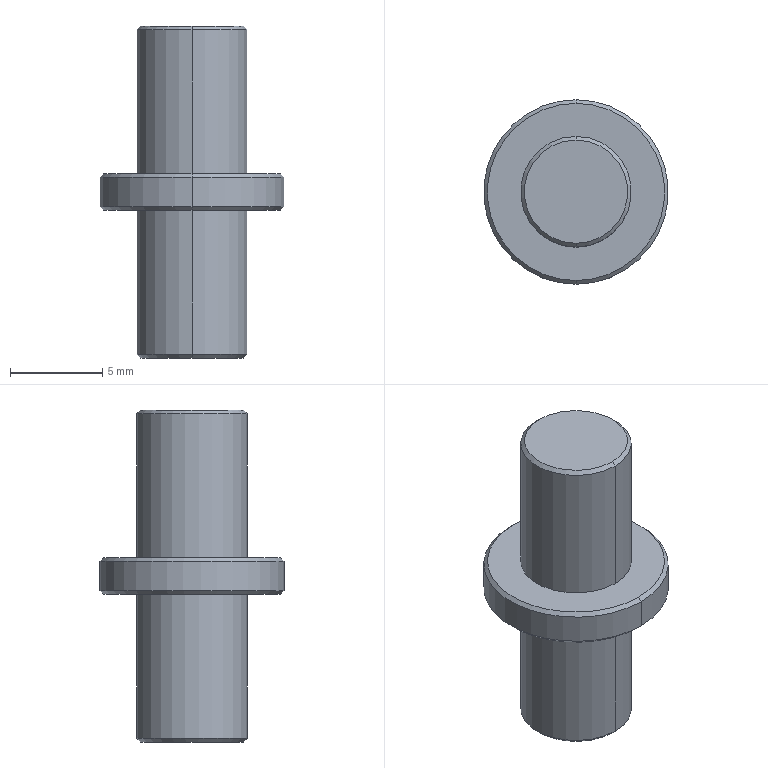Part | STEP file | RJWD-DY-0102_X2_5DE667DC95E8_24 | 1 solid | 18 faces | box 10 x 10 x 18 mm | volume 607.492 mm3 | cone 8 | cylinder 6 | plane 4 | commonest cylinder face diameters 6 x4 10 x2
STEP:
#1=CARTESIAN_POINT('',(0.,0.,0.));
#2=DIRECTION('',(0.,0.,1.));
#3=DIRECTION('',(1.,0.,0.));
#4=AXIS2_PLACEMENT_3D('',#1,#2,#3);
#5=CARTESIAN_POINT('',(-506.773,4252.873,40.144));
#6=VERTEX_POINT('',#5);
#7=CARTESIAN_POINT('',(-506.773,4247.273,40.144));
#8=VERTEX_POINT('',#7);
#9=CARTESIAN_POINT('',(-506.773,4250.073,40.144));
#10=DIRECTION('',(0.,0.,1.));
#11=DIRECTION('',(0.,1.,0.));
#12=AXIS2_PLACEMENT_3D('',#9,#10,#11);
#13=CIRCLE('',#12,2.8);
#14=CARTESIAN_POINT('',(-506.773,4250.073,40.144));
#15=DIRECTION('',(0.,0.,1.));
#16=DIRECTION('',(0.,1.,0.));
#17=AXIS2_PLACEMENT_3D('',#14,#15,#16);
#18=PLANE('',#17);
#19=CARTESIAN_POINT('',(0.,0.));
#20=DIRECTION('',(1.,0.));
#21=AXIS2_PLACEMENT_2D('',#19,#20);
#22=CIRCLE('',#21,2.8);
#23=(GEOMETRIC_REPRESENTATION_CONTEXT(2)PARAMETRIC_REPRESENTATION_CONTEXT()REPRESENTATION_CONTEXT('',''));
#24=DEFINITIONAL_REPRESENTATION('',(#22),#23);
#25=PCURVE('',#18,#24);
#26=CARTESIAN_POINT('',(-506.773,4250.073,40.044));
#27=DIRECTION('',(0.,0.,-1.));
#28=DIRECTION('',(0.,-1.,0.));
#29=AXIS2_PLACEMENT_3D('',#26,#27,#28);
#30=CONICAL_SURFACE('',#29,2.9,0.7854);
#31=CARTESIAN_POINT('',(3.142,-0.1));
#32=DIRECTION('',(-1.,0.));
#33=VECTOR('',#32,1.);
#34=LINE('',#31,#33);
#35=(GEOMETRIC_REPRESENTATION_CONTEXT(2)PARAMETRIC_REPRESENTATION_CONTEXT()REPRESENTATION_CONTEXT('',''));
#36=DEFINITIONAL_REPRESENTATION('',(#34),#35);
#37=PCURVE('',#30,#36);
#38=SURFACE_CURVE('',#13,(#25,#37),.PCURVE_S1.);
#39=EDGE_CURVE('',#6,#8,#38,.T.);
#40=ORIENTED_EDGE('',*,*,#39,.F.);
#41=CARTESIAN_POINT('',(-506.773,4250.073,40.144));
#42=DIRECTION('',(0.,0.,1.));
#43=DIRECTION('',(0.,-1.,0.));
#44=AXIS2_PLACEMENT_3D('',#41,#42,#43);
#45=CIRCLE('',#44,2.8);
#46=CARTESIAN_POINT('',(0.,0.));
#47=DIRECTION('',(-1.,0.));
#48=AXIS2_PLACEMENT_2D('',#46,#47);
#49=CIRCLE('',#48,2.8);
#50=(GEOMETRIC_REPRESENTATION_CONTEXT(2)PARAMETRIC_REPRESENTATION_CONTEXT()REPRESENTATION_CONTEXT('',''));
#51=DEFINITIONAL_REPRESENTATION('',(#49),#50);
#52=PCURVE('',#18,#51);
#53=CARTESIAN_POINT('',(-506.773,4250.073,40.044));
#54=DIRECTION('',(0.,0.,-1.));
#55=DIRECTION('',(0.,-1.,0.));
#56=AXIS2_PLACEMENT_3D('',#53,#54,#55);
#57=CONICAL_SURFACE('',#56,2.9,0.7854);
#58=CARTESIAN_POINT('',(6.283,-0.1));
#59=DIRECTION('',(-1.,0.));
#60=VECTOR('',#59,1.);
#61=LINE('',#58,#60);
#62=(GEOMETRIC_REPRESENTATION_CONTEXT(2)PARAMETRIC_REPRESENTATION_CONTEXT()REPRESENTATION_CONTEXT('',''));
#63=DEFINITIONAL_REPRESENTATION('',(#61),#62);
#64=PCURVE('',#57,#63);
#65=SURFACE_CURVE('',#45,(#52,#64),.PCURVE_S1.);
#66=EDGE_CURVE('',#8,#6,#65,.T.);
#67=ORIENTED_EDGE('',*,*,#66,.F.);
#68=EDGE_LOOP('',(#40,#67));
#69=FACE_BOUND('',#68,.F.);
#70=ADVANCED_FACE('',(#69),#18,.T.);
#71=ORIENTED_EDGE('',*,*,#39,.F.);
#72=CARTESIAN_POINT('',(-506.773,4253.073,39.944));
#73=VERTEX_POINT('',#72);
#74=CARTESIAN_POINT('',(-506.773,4252.873,40.144));
#75=DIRECTION('',(0.,0.7071,-0.7071));
#76=VECTOR('',#75,1.);
#77=LINE('',#74,#76);
#78=CARTESIAN_POINT('',(3.142,-0.1));
#79=DIRECTION('',(0.,1.));
#80=VECTOR('',#79,1.);
#81=LINE('',#78,#80);
#82=(GEOMETRIC_REPRESENTATION_CONTEXT(2)PARAMETRIC_REPRESENTATION_CONTEXT()REPRESENTATION_CONTEXT('',''));
#83=DEFINITIONAL_REPRESENTATION('',(#81),#82);
#84=PCURVE('',#30,#83);
#85=CARTESIAN_POINT('',(3.142,-0.1));
#86=DIRECTION('',(0.,1.));
#87=VECTOR('',#86,1.);
#88=LINE('',#85,#87);
#89=(GEOMETRIC_REPRESENTATION_CONTEXT(2)PARAMETRIC_REPRESENTATION_CONTEXT()REPRESENTATION_CONTEXT('',''));
#90=DEFINITIONAL_REPRESENTATION('',(#88),#89);
#91=PCURVE('',#57,#90);
#92=SURFACE_CURVE('',#77,(#84,#91),.PCURVE_S1.);
#93=EDGE_CURVE('',#6,#73,#92,.T.);
#94=ORIENTED_EDGE('',*,*,#93,.T.);
#95=CARTESIAN_POINT('',(-506.773,4247.073,39.944));
#96=VERTEX_POINT('',#95);
#97=CARTESIAN_POINT('',(-506.773,4250.073,39.944));
#98=DIRECTION('',(0.,0.,1.));
#99=DIRECTION('',(0.,1.,0.));
#100=AXIS2_PLACEMENT_3D('',#97,#98,#99);
#101=CIRCLE('',#100,3.);
#102=CARTESIAN_POINT('',(3.142,0.1));
#103=DIRECTION('',(-1.,0.));
#104=VECTOR('',#103,1.);
#105=LINE('',#102,#104);
#106=(GEOMETRIC_REPRESENTATION_CONTEXT(2)PARAMETRIC_REPRESENTATION_CONTEXT()REPRESENTATION_CONTEXT('',''));
#107=DEFINITIONAL_REPRESENTATION('',(#105),#106);
#108=PCURVE('',#30,#107);
#109=CARTESIAN_POINT('',(-506.773,4250.073,21.244));
#110=DIRECTION('',(0.,0.,1.));
#111=DIRECTION('',(0.,1.,0.));
#112=AXIS2_PLACEMENT_3D('',#109,#110,#111);
#113=CYLINDRICAL_SURFACE('',#112,3.);
#114=CARTESIAN_POINT('',(0.,18.7));
#115=DIRECTION('',(1.,0.));
#116=VECTOR('',#115,1.);
#117=LINE('',#114,#116);
#118=(GEOMETRIC_REPRESENTATION_CONTEXT(2)PARAMETRIC_REPRESENTATION_CONTEXT()REPRESENTATION_CONTEXT('',''));
#119=DEFINITIONAL_REPRESENTATION('',(#117),#118);
#120=PCURVE('',#113,#119);
#121=SURFACE_CURVE('',#101,(#108,#120),.PCURVE_S1.);
#122=EDGE_CURVE('',#73,#96,#121,.T.);
#123=ORIENTED_EDGE('',*,*,#122,.T.);
#124=CARTESIAN_POINT('',(-506.773,4247.273,40.144));
#125=DIRECTION('',(0.,-0.7071,-0.7071));
#126=VECTOR('',#125,1.);
#127=LINE('',#124,#126);
#128=CARTESIAN_POINT('',(0.,-0.1));
#129=DIRECTION('',(0.,1.));
#130=VECTOR('',#129,1.);
#131=LINE('',#128,#130);
#132=(GEOMETRIC_REPRESENTATION_CONTEXT(2)PARAMETRIC_REPRESENTATION_CONTEXT()REPRESENTATION_CONTEXT('',''));
#133=DEFINITIONAL_REPRESENTATION('',(#131),#132);
#134=PCURVE('',#30,#133);
#135=CARTESIAN_POINT('',(6.283,-0.1));
#136=DIRECTION('',(0.,1.));
#137=VECTOR('',#136,1.);
#138=LINE('',#135,#137);
#139=(GEOMETRIC_REPRESENTATION_CONTEXT(2)PARAMETRIC_REPRESENTATION_CONTEXT()REPRESENTATION_CONTEXT('',''));
#140=DEFINITIONAL_REPRESENTATION('',(#138),#139);
#141=PCURVE('',#57,#140);
#142=SURFACE_CURVE('',#127,(#134,#141),.PCURVE_S1.);
#143=EDGE_CURVE('',#8,#96,#142,.T.);
#144=ORIENTED_EDGE('',*,*,#143,.F.);
#145=EDGE_LOOP('',(#71,#94,#123,#144));
#146=FACE_BOUND('',#145,.T.);
#147=ADVANCED_FACE('',(#146),#30,.T.);
#148=ORIENTED_EDGE('',*,*,#66,.F.);
#149=ORIENTED_EDGE('',*,*,#143,.T.);
#150=CARTESIAN_POINT('',(-506.773,4250.073,39.944));
#151=DIRECTION('',(0.,0.,1.));
#152=DIRECTION('',(0.,-1.,0.));
#153=AXIS2_PLACEMENT_3D('',#150,#151,#152);
#154=CIRCLE('',#153,3.);
#155=CARTESIAN_POINT('',(6.283,0.1));
#156=DIRECTION('',(-1.,0.));
#157=VECTOR('',#156,1.);
#158=LINE('',#155,#157);
#159=(GEOMETRIC_REPRESENTATION_CONTEXT(2)PARAMETRIC_REPRESENTATION_CONTEXT()REPRESENTATION_CONTEXT('',''));
#160=DEFINITIONAL_REPRESENTATION('',(#158),#159);
#161=PCURVE('',#57,#160);
#162=CARTESIAN_POINT('',(-506.773,4250.073,21.244));
#163=DIRECTION('',(0.,0.,1.));
#164=DIRECTION('',(0.,1.,0.));
#165=AXIS2_PLACEMENT_3D('',#162,#163,#164);
#166=CYLINDRICAL_SURFACE('',#165,3.);
#167=CARTESIAN_POINT('',(3.142,18.7));
#168=DIRECTION('',(1.,0.));
#169=VECTOR('',#168,1.);
#170=LINE('',#167,#169);
#171=(GEOMETRIC_REPRESENTATION_CONTEXT(2)PARAMETRIC_REPRESENTATION_CONTEXT()REPRESENTATION_CONTEXT('',''));
#172=DEFINITIONAL_REPRESENTATION('',(#170),#171);
#173=PCURVE('',#166,#172);
#174=SURFACE_CURVE('',#154,(#161,#173),.PCURVE_S1.);
#175=EDGE_CURVE('',#96,#73,#174,.T.);
#176=ORIENTED_EDGE('',*,*,#175,.T.);
#177=ORIENTED_EDGE('',*,*,#93,.F.);
#178=EDGE_LOOP('',(#148,#149,#176,#177));
#179=FACE_BOUND('',#178,.T.);
#180=ADVANCED_FACE('',(#179),#57,.T.);
#181=CARTESIAN_POINT('',(-506.773,4253.073,32.144));
#182=VERTEX_POINT('',#181);
#183=CARTESIAN_POINT('',(-506.773,4247.073,32.144));
#184=VERTEX_POINT('',#183);
#185=CARTESIAN_POINT('',(-506.773,4250.073,32.144));
#186=DIRECTION('',(0.,0.,-1.));
#187=DIRECTION('',(0.,1.,0.));
#188=AXIS2_PLACEMENT_3D('',#185,#186,#187);
#189=CIRCLE('',#188,3.);
#190=CARTESIAN_POINT('',(6.283,10.9));
#191=DIRECTION('',(-1.,0.));
#192=VECTOR('',#191,1.);
#193=LINE('',#190,#192);
#194=(GEOMETRIC_REPRESENTATION_CONTEXT(2)PARAMETRIC_REPRESENTATION_CONTEXT()REPRESENTATION_CONTEXT('',''));
#195=DEFINITIONAL_REPRESENTATION('',(#193),#194);
#196=PCURVE('',#166,#195);
#197=CARTESIAN_POINT('',(-506.773,4250.073,32.144));
#198=DIRECTION('',(0.,0.,1.));
#199=DIRECTION('',(0.,1.,0.));
#200=AXIS2_PLACEMENT_3D('',#197,#198,#199);
#201=PLANE('',#200);
#202=CARTESIAN_POINT('',(3.,0.));
#203=CARTESIAN_POINT('',(3.,-5.196));
#204=CARTESIAN_POINT('',(-1.5,-2.598));
#205=CARTESIAN_POINT('',(-6.,0.));
#206=CARTESIAN_POINT('',(-1.5,2.598));
#207=CARTESIAN_POINT('',(3.,5.196));
#208=CARTESIAN_POINT('',(3.,0.));
#209=(BOUNDED_CURVE()B_SPLINE_CURVE(2,(#202,#203,#204,#205,#206,#207,#208),.UNSPECIFIED.,.T.,.F.)B_SPLINE_CURVE_WITH_KNOTS((1,2,2,2,2,1),(-2.094,0.,2.094,4.189,6.283,8.378),.UNSPECIFIED.)CURVE()GEOMETRIC_REPRESENTATION_ITEM()RATIONAL_B_SPLINE_CURVE((1.,0.5,1.,0.5,1.,0.5,1.))REPRESENTATION_ITEM(''));
#210=(GEOMETRIC_REPRESENTATION_CONTEXT(2)PARAMETRIC_REPRESENTATION_CONTEXT()REPRESENTATION_CONTEXT('',''));
#211=DEFINITIONAL_REPRESENTATION('',(#209),#210);
#212=PCURVE('',#201,#211);
#213=SURFACE_CURVE('',#189,(#196,#212),.PCURVE_S1.);
#214=EDGE_CURVE('',#182,#184,#213,.T.);
#215=ORIENTED_EDGE('',*,*,#214,.F.);
#216=CARTESIAN_POINT('',(-506.773,4253.073,32.144));
#217=DIRECTION('',(0.,0.,1.));
#218=VECTOR('',#217,1.);
#219=LINE('',#216,#218);
#220=CARTESIAN_POINT('',(6.283,10.9));
#221=DIRECTION('',(0.,1.));
#222=VECTOR('',#221,1.);
#223=LINE('',#220,#222);
#224=(GEOMETRIC_REPRESENTATION_CONTEXT(2)PARAMETRIC_REPRESENTATION_CONTEXT()REPRESENTATION_CONTEXT('',''));
#225=DEFINITIONAL_REPRESENTATION('',(#223),#224);
#226=PCURVE('',#166,#225);
#227=CARTESIAN_POINT('',(0.,10.9));
#228=DIRECTION('',(0.,1.));
#229=VECTOR('',#228,1.);
#230=LINE('',#227,#229);
#231=(GEOMETRIC_REPRESENTATION_CONTEXT(2)PARAMETRIC_REPRESENTATION_CONTEXT()REPRESENTATION_CONTEXT('',''));
#232=DEFINITIONAL_REPRESENTATION('',(#230),#231);
#233=PCURVE('',#113,#232);
#234=SURFACE_CURVE('',#219,(#226,#233),.PCURVE_S1.);
#235=EDGE_CURVE('',#182,#73,#234,.T.);
#236=ORIENTED_EDGE('',*,*,#235,.T.);
#237=ORIENTED_EDGE('',*,*,#175,.F.);
#238=CARTESIAN_POINT('',(-506.773,4247.073,32.144));
#239=DIRECTION('',(0.,0.,1.));
#240=VECTOR('',#239,1.);
#241=LINE('',#238,#240);
#242=CARTESIAN_POINT('',(3.142,10.9));
#243=DIRECTION('',(0.,1.));
#244=VECTOR('',#243,1.);
#245=LINE('',#242,#244);
#246=(GEOMETRIC_REPRESENTATION_CONTEXT(2)PARAMETRIC_REPRESENTATION_CONTEXT()REPRESENTATION_CONTEXT('',''));
#247=DEFINITIONAL_REPRESENTATION('',(#245),#246);
#248=PCURVE('',#166,#247);
#249=CARTESIAN_POINT('',(3.142,10.9));
#250=DIRECTION('',(0.,1.));
#251=VECTOR('',#250,1.);
#252=LINE('',#249,#251);
#253=(GEOMETRIC_REPRESENTATION_CONTEXT(2)PARAMETRIC_REPRESENTATION_CONTEXT()REPRESENTATION_CONTEXT('',''));
#254=DEFINITIONAL_REPRESENTATION('',(#252),#253);
#255=PCURVE('',#113,#254);
#256=SURFACE_CURVE('',#241,(#248,#255),.PCURVE_S1.);
#257=EDGE_CURVE('',#184,#96,#256,.T.);
#258=ORIENTED_EDGE('',*,*,#257,.F.);
#259=EDGE_LOOP('',(#215,#236,#237,#258));
#260=FACE_BOUND('',#259,.T.);
#261=ADVANCED_FACE('',(#260),#166,.T.);
#262=CARTESIAN_POINT('',(-506.773,4250.073,32.144));
#263=DIRECTION('',(0.,0.,-1.));
#264=DIRECTION('',(0.,-1.,0.));
#265=AXIS2_PLACEMENT_3D('',#262,#263,#264);
#266=CIRCLE('',#265,3.);
#267=CARTESIAN_POINT('',(3.142,10.9));
#268=DIRECTION('',(-1.,0.));
#269=VECTOR('',#268,1.);
#270=LINE('',#267,#269);
#271=(GEOMETRIC_REPRESENTATION_CONTEXT(2)PARAMETRIC_REPRESENTATION_CONTEXT()REPRESENTATION_CONTEXT('',''));
#272=DEFINITIONAL_REPRESENTATION('',(#270),#271);
#273=PCURVE('',#113,#272);
#274=CARTESIAN_POINT('',(-3.,0.));
#275=CARTESIAN_POINT('',(-3.,5.196));
#276=CARTESIAN_POINT('',(1.5,2.598));
#277=CARTESIAN_POINT('',(6.,0.));
#278=CARTESIAN_POINT('',(1.5,-2.598));
#279=CARTESIAN_POINT('',(-3.,-5.196));
#280=CARTESIAN_POINT('',(-3.,0.));
#281=(BOUNDED_CURVE()B_SPLINE_CURVE(2,(#274,#275,#276,#277,#278,#279,#280),.UNSPECIFIED.,.T.,.F.)B_SPLINE_CURVE_WITH_KNOTS((1,2,2,2,2,1),(-2.094,0.,2.094,4.189,6.283,8.378),.UNSPECIFIED.)CURVE()GEOMETRIC_REPRESENTATION_ITEM()RATIONAL_B_SPLINE_CURVE((1.,0.5,1.,0.5,1.,0.5,1.))REPRESENTATION_ITEM(''));
#282=(GEOMETRIC_REPRESENTATION_CONTEXT(2)PARAMETRIC_REPRESENTATION_CONTEXT()REPRESENTATION_CONTEXT('',''));
#283=DEFINITIONAL_REPRESENTATION('',(#281),#282);
#284=PCURVE('',#201,#283);
#285=SURFACE_CURVE('',#266,(#273,#284),.PCURVE_S1.);
#286=EDGE_CURVE('',#184,#182,#285,.T.);
#287=ORIENTED_EDGE('',*,*,#286,.F.);
#288=ORIENTED_EDGE('',*,*,#257,.T.);
#289=ORIENTED_EDGE('',*,*,#122,.F.);
#290=ORIENTED_EDGE('',*,*,#235,.F.);
#291=EDGE_LOOP('',(#287,#288,#289,#290));
#292=FACE_BOUND('',#291,.T.);
#293=ADVANCED_FACE('',(#292),#113,.T.);
#294=CARTESIAN_POINT('',(-506.773,4254.873,32.144));
#295=VERTEX_POINT('',#294);
#296=CARTESIAN_POINT('',(-506.773,4245.273,32.144));
#297=VERTEX_POINT('',#296);
#298=CARTESIAN_POINT('',(-506.773,4250.073,32.144));
#299=DIRECTION('',(0.,0.,1.));
#300=DIRECTION('',(0.,1.,0.));
#301=AXIS2_PLACEMENT_3D('',#298,#299,#300);
#302=CIRCLE('',#301,4.8);
#303=CARTESIAN_POINT('',(0.,0.));
#304=DIRECTION('',(1.,0.));
#305=AXIS2_PLACEMENT_2D('',#303,#304);
#306=CIRCLE('',#305,4.8);
#307=(GEOMETRIC_REPRESENTATION_CONTEXT(2)PARAMETRIC_REPRESENTATION_CONTEXT()REPRESENTATION_CONTEXT('',''));
#308=DEFINITIONAL_REPRESENTATION('',(#306),#307);
#309=PCURVE('',#201,#308);
#310=CARTESIAN_POINT('',(-506.773,4250.073,32.044));
#311=DIRECTION('',(0.,0.,-1.));
#312=DIRECTION('',(0.,-1.,0.));
#313=AXIS2_PLACEMENT_3D('',#310,#311,#312);
#314=CONICAL_SURFACE('',#313,4.9,0.7854);
#315=CARTESIAN_POINT('',(3.142,-0.1));
#316=DIRECTION('',(-1.,0.));
#317=VECTOR('',#316,1.);
#318=LINE('',#315,#317);
#319=(GEOMETRIC_REPRESENTATION_CONTEXT(2)PARAMETRIC_REPRESENTATION_CONTEXT()REPRESENTATION_CONTEXT('',''));
#320=DEFINITIONAL_REPRESENTATION('',(#318),#319);
#321=PCURVE('',#314,#320);
#322=SURFACE_CURVE('',#302,(#309,#321),.PCURVE_S1.);
#323=EDGE_CURVE('',#295,#297,#322,.T.);
#324=ORIENTED_EDGE('',*,*,#323,.F.);
#325=CARTESIAN_POINT('',(-506.773,4250.073,32.144));
#326=DIRECTION('',(0.,0.,1.));
#327=DIRECTION('',(0.,-1.,0.));
#328=AXIS2_PLACEMENT_3D('',#325,#326,#327);
#329=CIRCLE('',#328,4.8);
#330=CARTESIAN_POINT('',(0.,0.));
#331=DIRECTION('',(-1.,0.));
#332=AXIS2_PLACEMENT_2D('',#330,#331);
#333=CIRCLE('',#332,4.8);
#334=(GEOMETRIC_REPRESENTATION_CONTEXT(2)PARAMETRIC_REPRESENTATION_CONTEXT()REPRESENTATION_CONTEXT('',''));
#335=DEFINITIONAL_REPRESENTATION('',(#333),#334);
#336=PCURVE('',#201,#335);
#337=CARTESIAN_POINT('',(-506.773,4250.073,32.044));
#338=DIRECTION('',(0.,0.,-1.));
#339=DIRECTION('',(0.,-1.,0.));
#340=AXIS2_PLACEMENT_3D('',#337,#338,#339);
#341=CONICAL_SURFACE('',#340,4.9,0.7854);
#342=CARTESIAN_POINT('',(6.283,-0.1));
#343=DIRECTION('',(-1.,0.));
#344=VECTOR('',#343,1.);
#345=LINE('',#342,#344);
#346=(GEOMETRIC_REPRESENTATION_CONTEXT(2)PARAMETRIC_REPRESENTATION_CONTEXT()REPRESENTATION_CONTEXT('',''));
#347=DEFINITIONAL_REPRESENTATION('',(#345),#346);
#348=PCURVE('',#341,#347);
#349=SURFACE_CURVE('',#329,(#336,#348),.PCURVE_S1.);
#350=EDGE_CURVE('',#297,#295,#349,.T.);
#351=ORIENTED_EDGE('',*,*,#350,.F.);
#352=EDGE_LOOP('',(#324,#351));
#353=FACE_BOUND('',#352,.F.);
#354=ORIENTED_EDGE('',*,*,#214,.F.);
#355=ORIENTED_EDGE('',*,*,#286,.F.);
#356=EDGE_LOOP('',(#354,#355));
#357=FACE_BOUND('',#356,.F.);
#358=ADVANCED_FACE('',(#353,#357),#201,.T.);
#359=ORIENTED_EDGE('',*,*,#323,.F.);
#360=CARTESIAN_POINT('',(-506.773,4255.073,31.944));
#361=VERTEX_POINT('',#360);
#362=CARTESIAN_POINT('',(-506.773,4254.873,32.144));
#363=DIRECTION('',(0.,0.7071,-0.7071));
#364=VECTOR('',#363,1.);
#365=LINE('',#362,#364);
#366=CARTESIAN_POINT('',(3.142,-0.1));
#367=DIRECTION('',(0.,1.));
#368=VECTOR('',#367,1.);
#369=LINE('',#366,#368);
#370=(GEOMETRIC_REPRESENTATION_CONTEXT(2)PARAMETRIC_REPRESENTATION_CONTEXT()REPRESENTATION_CONTEXT('',''));
#371=DEFINITIONAL_REPRESENTATION('',(#369),#370);
#372=PCURVE('',#314,#371);
#373=CARTESIAN_POINT('',(3.142,-0.1));
#374=DIRECTION('',(0.,1.));
#375=VECTOR('',#374,1.);
#376=LINE('',#373,#375);
#377=(GEOMETRIC_REPRESENTATION_CONTEXT(2)PARAMETRIC_REPRESENTATION_CONTEXT()REPRESENTATION_CONTEXT('',''));
#378=DEFINITIONAL_REPRESENTATION('',(#376),#377);
#379=PCURVE('',#341,#378);
#380=SURFACE_CURVE('',#365,(#372,#379),.PCURVE_S1.);
#381=EDGE_CURVE('',#295,#361,#380,.T.);
#382=ORIENTED_EDGE('',*,*,#381,.T.);
#383=CARTESIAN_POINT('',(-506.773,4245.073,31.944));
#384=VERTEX_POINT('',#383);
#385=CARTESIAN_POINT('',(-506.773,4250.073,31.944));
#386=DIRECTION('',(0.,0.,1.));
#387=DIRECTION('',(0.,1.,0.));
#388=AXIS2_PLACEMENT_3D('',#385,#386,#387);
#389=CIRCLE('',#388,5.);
#390=CARTESIAN_POINT('',(3.142,0.1));
#391=DIRECTION('',(-1.,0.));
#392=VECTOR('',#391,1.);
#393=LINE('',#390,#392);
#394=(GEOMETRIC_REPRESENTATION_CONTEXT(2)PARAMETRIC_REPRESENTATION_CONTEXT()REPRESENTATION_CONTEXT('',''));
#395=DEFINITIONAL_REPRESENTATION('',(#393),#394);
#396=PCURVE('',#314,#395);
#397=CARTESIAN_POINT('',(-506.773,4250.073,21.244));
#398=DIRECTION('',(0.,0.,1.));
#399=DIRECTION('',(0.,1.,0.));
#400=AXIS2_PLACEMENT_3D('',#397,#398,#399);
#401=CYLINDRICAL_SURFACE('',#400,5.);
#402=CARTESIAN_POINT('',(0.,10.7));
#403=DIRECTION('',(1.,0.));
#404=VECTOR('',#403,1.);
#405=LINE('',#402,#404);
#406=(GEOMETRIC_REPRESENTATION_CONTEXT(2)PARAMETRIC_REPRESENTATION_CONTEXT()REPRESENTATION_CONTEXT('',''));
#407=DEFINITIONAL_REPRESENTATION('',(#405),#406);
#408=PCURVE('',#401,#407);
#409=SURFACE_CURVE('',#389,(#396,#408),.PCURVE_S1.);
#410=EDGE_CURVE('',#361,#384,#409,.T.);
#411=ORIENTED_EDGE('',*,*,#410,.T.);
#412=CARTESIAN_POINT('',(-506.773,4245.273,32.144));
#413=DIRECTION('',(0.,-0.7071,-0.7071));
#414=VECTOR('',#413,1.);
#415=LINE('',#412,#414);
#416=CARTESIAN_POINT('',(0.,-0.1));
#417=DIRECTION('',(0.,1.));
#418=VECTOR('',#417,1.);
#419=LINE('',#416,#418);
#420=(GEOMETRIC_REPRESENTATION_CONTEXT(2)PARAMETRIC_REPRESENTATION_CONTEXT()REPRESENTATION_CONTEXT('',''));
#421=DEFINITIONAL_REPRESENTATION('',(#419),#420);
#422=PCURVE('',#314,#421);
#423=CARTESIAN_POINT('',(6.283,-0.1));
#424=DIRECTION('',(0.,1.));
#425=VECTOR('',#424,1.);
#426=LINE('',#423,#425);
#427=(GEOMETRIC_REPRESENTATION_CONTEXT(2)PARAMETRIC_REPRESENTATION_CONTEXT()REPRESENTATION_CONTEXT('',''));
#428=DEFINITIONAL_REPRESENTATION('',(#426),#427);
#429=PCURVE('',#341,#428);
#430=SURFACE_CURVE('',#415,(#422,#429),.PCURVE_S1.);
#431=EDGE_CURVE('',#297,#384,#430,.T.);
#432=ORIENTED_EDGE('',*,*,#431,.F.);
#433=EDGE_LOOP('',(#359,#382,#411,#432));
#434=FACE_BOUND('',#433,.T.);
#435=ADVANCED_FACE('',(#434),#314,.T.);
#436=ORIENTED_EDGE('',*,*,#350,.F.);
#437=ORIENTED_EDGE('',*,*,#431,.T.);
#438=CARTESIAN_POINT('',(-506.773,4250.073,31.944));
#439=DIRECTION('',(0.,0.,1.));
#440=DIRECTION('',(0.,-1.,0.));
#441=AXIS2_PLACEMENT_3D('',#438,#439,#440);
#442=CIRCLE('',#441,5.);
#443=CARTESIAN_POINT('',(6.283,0.1));
#444=DIRECTION('',(-1.,0.));
#445=VECTOR('',#444,1.);
#446=LINE('',#443,#445);
#447=(GEOMETRIC_REPRESENTATION_CONTEXT(2)PARAMETRIC_REPRESENTATION_CONTEXT()REPRESENTATION_CONTEXT('',''));
#448=DEFINITIONAL_REPRESENTATION('',(#446),#447);
#449=PCURVE('',#341,#448);
#450=CARTESIAN_POINT('',(-506.773,4250.073,21.244));
#451=DIRECTION('',(0.,0.,1.));
#452=DIRECTION('',(0.,1.,0.));
#453=AXIS2_PLACEMENT_3D('',#450,#451,#452);
#454=CYLINDRICAL_SURFACE('',#453,5.);
#455=CARTESIAN_POINT('',(3.142,10.7));
#456=DIRECTION('',(1.,0.));
#457=VECTOR('',#456,1.);
#458=LINE('',#455,#457);
#459=(GEOMETRIC_REPRESENTATION_CONTEXT(2)PARAMETRIC_REPRESENTATION_CONTEXT()REPRESENTATION_CONTEXT('',''));
#460=DEFINITIONAL_REPRESENTATION('',(#458),#459);
#461=PCURVE('',#454,#460);
#462=SURFACE_CURVE('',#442,(#449,#461),.PCURVE_S1.);
#463=EDGE_CURVE('',#384,#361,#462,.T.);
#464=ORIENTED_EDGE('',*,*,#463,.T.);
#465=ORIENTED_EDGE('',*,*,#381,.F.);
#466=EDGE_LOOP('',(#436,#437,#464,#465));
#467=FACE_BOUND('',#466,.T.);
#468=ADVANCED_FACE('',(#467),#341,.T.);
#469=ORIENTED_EDGE('',*,*,#463,.F.);
#470=CARTESIAN_POINT('',(-506.773,4245.073,30.344));
#471=VERTEX_POINT('',#470);
#472=CARTESIAN_POINT('',(-506.773,4245.073,30.344));
#473=DIRECTION('',(0.,0.,1.));
#474=VECTOR('',#473,1.);
#475=LINE('',#472,#474);
#476=CARTESIAN_POINT('',(3.142,9.1));
#477=DIRECTION('',(0.,1.));
#478=VECTOR('',#477,1.);
#479=LINE('',#476,#478);
#480=(GEOMETRIC_REPRESENTATION_CONTEXT(2)PARAMETRIC_REPRESENTATION_CONTEXT()REPRESENTATION_CONTEXT('',''));
#481=DEFINITIONAL_REPRESENTATION('',(#479),#480);
#482=PCURVE('',#454,#481);
#483=CARTESIAN_POINT('',(3.142,9.1));
#484=DIRECTION('',(0.,1.));
#485=VECTOR('',#484,1.);
#486=LINE('',#483,#485);
#487=(GEOMETRIC_REPRESENTATION_CONTEXT(2)PARAMETRIC_REPRESENTATION_CONTEXT()REPRESENTATION_CONTEXT('',''));
#488=DEFINITIONAL_REPRESENTATION('',(#486),#487);
#489=PCURVE('',#401,#488);
#490=SURFACE_CURVE('',#475,(#482,#489),.PCURVE_S1.);
#491=EDGE_CURVE('',#471,#384,#490,.T.);
#492=ORIENTED_EDGE('',*,*,#491,.F.);
#493=CARTESIAN_POINT('',(-506.773,4255.073,30.344));
#494=VERTEX_POINT('',#493);
#495=CARTESIAN_POINT('',(-506.773,4250.073,30.344));
#496=DIRECTION('',(0.,0.,-1.));
#497=DIRECTION('',(0.,1.,0.));
#498=AXIS2_PLACEMENT_3D('',#495,#496,#497);
#499=CIRCLE('',#498,5.);
#500=CARTESIAN_POINT('',(6.283,9.1));
#501=DIRECTION('',(-1.,0.));
#502=VECTOR('',#501,1.);
#503=LINE('',#500,#502);
#504=(GEOMETRIC_REPRESENTATION_CONTEXT(2)PARAMETRIC_REPRESENTATION_CONTEXT()REPRESENTATION_CONTEXT('',''));
#505=DEFINITIONAL_REPRESENTATION('',(#503),#504);
#506=PCURVE('',#454,#505);
#507=CARTESIAN_POINT('',(-506.773,4250.073,30.244));
#508=DIRECTION('',(0.,0.,1.));
#509=DIRECTION('',(0.,-1.,0.));
#510=AXIS2_PLACEMENT_3D('',#507,#508,#509);
#511=CONICAL_SURFACE('',#510,4.9,0.7854);
#512=CARTESIAN_POINT('',(3.142,0.1));
#513=DIRECTION('',(-1.,0.));
#514=VECTOR('',#513,1.);
#515=LINE('',#512,#514);
#516=(GEOMETRIC_REPRESENTATION_CONTEXT(2)PARAMETRIC_REPRESENTATION_CONTEXT()REPRESENTATION_CONTEXT('',''));
#517=DEFINITIONAL_REPRESENTATION('',(#515),#516);
#518=PCURVE('',#511,#517);
#519=SURFACE_CURVE('',#499,(#506,#518),.PCURVE_S1.);
#520=EDGE_CURVE('',#494,#471,#519,.T.);
#521=ORIENTED_EDGE('',*,*,#520,.F.);
#522=CARTESIAN_POINT('',(-506.773,4255.073,30.344));
#523=DIRECTION('',(0.,0.,1.));
#524=VECTOR('',#523,1.);
#525=LINE('',#522,#524);
#526=CARTESIAN_POINT('',(6.283,9.1));
#527=DIRECTION('',(0.,1.));
#528=VECTOR('',#527,1.);
#529=LINE('',#526,#528);
#530=(GEOMETRIC_REPRESENTATION_CONTEXT(2)PARAMETRIC_REPRESENTATION_CONTEXT()REPRESENTATION_CONTEXT('',''));
#531=DEFINITIONAL_REPRESENTATION('',(#529),#530);
#532=PCURVE('',#454,#531);
#533=CARTESIAN_POINT('',(0.,9.1));
#534=DIRECTION('',(0.,1.));
#535=VECTOR('',#534,1.);
#536=LINE('',#533,#535);
#537=(GEOMETRIC_REPRESENTATION_CONTEXT(2)PARAMETRIC_REPRESENTATION_CONTEXT()REPRESENTATION_CONTEXT('',''));
#538=DEFINITIONAL_REPRESENTATION('',(#536),#537);
#539=PCURVE('',#401,#538);
#540=SURFACE_CURVE('',#525,(#532,#539),.PCURVE_S1.);
#541=EDGE_CURVE('',#494,#361,#540,.T.);
#542=ORIENTED_EDGE('',*,*,#541,.T.);
#543=EDGE_LOOP('',(#469,#492,#521,#542));
#544=FACE_BOUND('',#543,.T.);
#545=ADVANCED_FACE('',(#544),#454,.T.);
#546=ORIENTED_EDGE('',*,*,#410,.F.);
#547=ORIENTED_EDGE('',*,*,#541,.F.);
#548=CARTESIAN_POINT('',(-506.773,4250.073,30.344));
#549=DIRECTION('',(0.,0.,-1.));
#550=DIRECTION('',(0.,-1.,0.));
#551=AXIS2_PLACEMENT_3D('',#548,#549,#550);
#552=CIRCLE('',#551,5.);
#553=CARTESIAN_POINT('',(3.142,9.1));
#554=DIRECTION('',(-1.,0.));
#555=VECTOR('',#554,1.);
#556=LINE('',#553,#555);
#557=(GEOMETRIC_REPRESENTATION_CONTEXT(2)PARAMETRIC_REPRESENTATION_CONTEXT()REPRESENTATION_CONTEXT('',''));
#558=DEFINITIONAL_REPRESENTATION('',(#556),#557);
#559=PCURVE('',#401,#558);
#560=CARTESIAN_POINT('',(-506.773,4250.073,30.244));
#561=DIRECTION('',(0.,0.,1.));
#562=DIRECTION('',(0.,-1.,0.));
#563=AXIS2_PLACEMENT_3D('',#560,#561,#562);
#564=CONICAL_SURFACE('',#563,4.9,0.7854);
#565=CARTESIAN_POINT('',(6.283,0.1));
#566=DIRECTION('',(-1.,0.));
#567=VECTOR('',#566,1.);
#568=LINE('',#565,#567);
#569=(GEOMETRIC_REPRESENTATION_CONTEXT(2)PARAMETRIC_REPRESENTATION_CONTEXT()REPRESENTATION_CONTEXT('',''));
#570=DEFINITIONAL_REPRESENTATION('',(#568),#569);
#571=PCURVE('',#564,#570);
#572=SURFACE_CURVE('',#552,(#559,#571),.PCURVE_S1.);
#573=EDGE_CURVE('',#471,#494,#572,.T.);
#574=ORIENTED_EDGE('',*,*,#573,.F.);
#575=ORIENTED_EDGE('',*,*,#491,.T.);
#576=EDGE_LOOP('',(#546,#547,#574,#575));
#577=FACE_BOUND('',#576,.T.);
#578=ADVANCED_FACE('',(#577),#401,.T.);
#579=ORIENTED_EDGE('',*,*,#573,.T.);
#580=CARTESIAN_POINT('',(-506.773,4254.873,30.144));
#581=VERTEX_POINT('',#580);
#582=CARTESIAN_POINT('',(-506.773,4255.073,30.344));
#583=DIRECTION('',(0.,-0.7071,-0.7071));
#584=VECTOR('',#583,1.);
#585=LINE('',#582,#584);
#586=CARTESIAN_POINT('',(3.142,0.1));
#587=DIRECTION('',(0.,-1.));
#588=VECTOR('',#587,1.);
#589=LINE('',#586,#588);
#590=(GEOMETRIC_REPRESENTATION_CONTEXT(2)PARAMETRIC_REPRESENTATION_CONTEXT()REPRESENTATION_CONTEXT('',''));
#591=DEFINITIONAL_REPRESENTATION('',(#589),#590);
#592=PCURVE('',#564,#591);
#593=CARTESIAN_POINT('',(3.142,0.1));
#594=DIRECTION('',(0.,-1.));
#595=VECTOR('',#594,1.);
#596=LINE('',#593,#595);
#597=(GEOMETRIC_REPRESENTATION_CONTEXT(2)PARAMETRIC_REPRESENTATION_CONTEXT()REPRESENTATION_CONTEXT('',''));
#598=DEFINITIONAL_REPRESENTATION('',(#596),#597);
#599=PCURVE('',#511,#598);
#600=SURFACE_CURVE('',#585,(#592,#599),.PCURVE_S1.);
#601=EDGE_CURVE('',#494,#581,#600,.T.);
#602=ORIENTED_EDGE('',*,*,#601,.T.);
#603=CARTESIAN_POINT('',(-506.773,4245.273,30.144));
#604=VERTEX_POINT('',#603);
#605=CARTESIAN_POINT('',(-506.773,4250.073,30.144));
#606=DIRECTION('',(0.,0.,-1.));
#607=DIRECTION('',(0.,-1.,0.));
#608=AXIS2_PLACEMENT_3D('',#605,#606,#607);
#609=CIRCLE('',#608,4.8);
#610=CARTESIAN_POINT('',(6.283,-0.1));
#611=DIRECTION('',(-1.,0.));
#612=VECTOR('',#611,1.);
#613=LINE('',#610,#612);
#614=(GEOMETRIC_REPRESENTATION_CONTEXT(2)PARAMETRIC_REPRESENTATION_CONTEXT()REPRESENTATION_CONTEXT('',''));
#615=DEFINITIONAL_REPRESENTATION('',(#613),#614);
#616=PCURVE('',#564,#615);
#617=CARTESIAN_POINT('',(-506.773,4250.073,30.144));
#618=DIRECTION('',(0.,0.,1.));
#619=DIRECTION('',(0.,1.,0.));
#620=AXIS2_PLACEMENT_3D('',#617,#618,#619);
#621=PLANE('',#620);
#622=CARTESIAN_POINT('',(-4.8,0.));
#623=CARTESIAN_POINT('',(-4.8,8.314));
#624=CARTESIAN_POINT('',(2.4,4.157));
#625=CARTESIAN_POINT('',(9.6,0.));
#626=CARTESIAN_POINT('',(2.4,-4.157));
#627=CARTESIAN_POINT('',(-4.8,-8.314));
#628=CARTESIAN_POINT('',(-4.8,0.));
#629=(BOUNDED_CURVE()B_SPLINE_CURVE(2,(#622,#623,#624,#625,#626,#627,#628),.UNSPECIFIED.,.T.,.F.)B_SPLINE_CURVE_WITH_KNOTS((1,2,2,2,2,1),(-2.094,0.,2.094,4.189,6.283,8.378),.UNSPECIFIED.)CURVE()GEOMETRIC_REPRESENTATION_ITEM()RATIONAL_B_SPLINE_CURVE((1.,0.5,1.,0.5,1.,0.5,1.))REPRESENTATION_ITEM(''));
#630=(GEOMETRIC_REPRESENTATION_CONTEXT(2)PARAMETRIC_REPRESENTATION_CONTEXT()REPRESENTATION_CONTEXT('',''));
#631=DEFINITIONAL_REPRESENTATION('',(#629),#630);
#632=PCURVE('',#621,#631);
#633=SURFACE_CURVE('',#609,(#616,#632),.PCURVE_S1.);
#634=EDGE_CURVE('',#604,#581,#633,.T.);
#635=ORIENTED_EDGE('',*,*,#634,.F.);
#636=CARTESIAN_POINT('',(-506.773,4245.073,30.344));
#637=DIRECTION('',(0.,0.7071,-0.7071));
#638=VECTOR('',#637,1.);
#639=LINE('',#636,#638);
#640=CARTESIAN_POINT('',(6.283,0.1));
#641=DIRECTION('',(0.,-1.));
#642=VECTOR('',#641,1.);
#643=LINE('',#640,#642);
#644=(GEOMETRIC_REPRESENTATION_CONTEXT(2)PARAMETRIC_REPRESENTATION_CONTEXT()REPRESENTATION_CONTEXT('',''));
#645=DEFINITIONAL_REPRESENTATION('',(#643),#644);
#646=PCURVE('',#564,#645);
#647=CARTESIAN_POINT('',(0.,0.1));
#648=DIRECTION('',(0.,-1.));
#649=VECTOR('',#648,1.);
#650=LINE('',#647,#649);
#651=(GEOMETRIC_REPRESENTATION_CONTEXT(2)PARAMETRIC_REPRESENTATION_CONTEXT()REPRESENTATION_CONTEXT('',''));
#652=DEFINITIONAL_REPRESENTATION('',(#650),#651);
#653=PCURVE('',#511,#652);
#654=SURFACE_CURVE('',#639,(#646,#653),.PCURVE_S1.);
#655=EDGE_CURVE('',#471,#604,#654,.T.);
#656=ORIENTED_EDGE('',*,*,#655,.F.);
#657=EDGE_LOOP('',(#579,#602,#635,#656));
#658=FACE_BOUND('',#657,.T.);
#659=ADVANCED_FACE('',(#658),#564,.T.);
#660=ORIENTED_EDGE('',*,*,#520,.T.);
#661=ORIENTED_EDGE('',*,*,#655,.T.);
#662=CARTESIAN_POINT('',(-506.773,4250.073,30.144));
#663=DIRECTION('',(0.,0.,-1.));
#664=DIRECTION('',(0.,1.,0.));
#665=AXIS2_PLACEMENT_3D('',#662,#663,#664);
#666=CIRCLE('',#665,4.8);
#667=CARTESIAN_POINT('',(3.142,-0.1));
#668=DIRECTION('',(-1.,0.));
#669=VECTOR('',#668,1.);
#670=LINE('',#667,#669);
#671=(GEOMETRIC_REPRESENTATION_CONTEXT(2)PARAMETRIC_REPRESENTATION_CONTEXT()REPRESENTATION_CONTEXT('',''));
#672=DEFINITIONAL_REPRESENTATION('',(#670),#671);
#673=PCURVE('',#511,#672);
#674=CARTESIAN_POINT('',(4.8,0.));
#675=CARTESIAN_POINT('',(4.8,-8.314));
#676=CARTESIAN_POINT('',(-2.4,-4.157));
#677=CARTESIAN_POINT('',(-9.6,0.));
#678=CARTESIAN_POINT('',(-2.4,4.157));
#679=CARTESIAN_POINT('',(4.8,8.314));
#680=CARTESIAN_POINT('',(4.8,0.));
#681=(BOUNDED_CURVE()B_SPLINE_CURVE(2,(#674,#675,#676,#677,#678,#679,#680),.UNSPECIFIED.,.T.,.F.)B_SPLINE_CURVE_WITH_KNOTS((1,2,2,2,2,1),(-2.094,0.,2.094,4.189,6.283,8.378),.UNSPECIFIED.)CURVE()GEOMETRIC_REPRESENTATION_ITEM()RATIONAL_B_SPLINE_CURVE((1.,0.5,1.,0.5,1.,0.5,1.))REPRESENTATION_ITEM(''));
#682=(GEOMETRIC_REPRESENTATION_CONTEXT(2)PARAMETRIC_REPRESENTATION_CONTEXT()REPRESENTATION_CONTEXT('',''));
#683=DEFINITIONAL_REPRESENTATION('',(#681),#682);
#684=PCURVE('',#621,#683);
#685=SURFACE_CURVE('',#666,(#673,#684),.PCURVE_S1.);
#686=EDGE_CURVE('',#581,#604,#685,.T.);
#687=ORIENTED_EDGE('',*,*,#686,.F.);
#688=ORIENTED_EDGE('',*,*,#601,.F.);
#689=EDGE_LOOP('',(#660,#661,#687,#688));
#690=FACE_BOUND('',#689,.T.);
#691=ADVANCED_FACE('',(#690),#511,.T.);
#692=ORIENTED_EDGE('',*,*,#634,.F.);
#693=ORIENTED_EDGE('',*,*,#686,.F.);
#694=EDGE_LOOP('',(#692,#693));
#695=FACE_BOUND('',#694,.F.);
#696=CARTESIAN_POINT('',(-506.773,4253.073,30.144));
#697=VERTEX_POINT('',#696);
#698=CARTESIAN_POINT('',(-506.773,4247.073,30.144));
#699=VERTEX_POINT('',#698);
#700=CARTESIAN_POINT('',(-506.773,4250.073,30.144));
#701=DIRECTION('',(0.,0.,1.));
#702=DIRECTION('',(0.,1.,0.));
#703=AXIS2_PLACEMENT_3D('',#700,#701,#702);
#704=CIRCLE('',#703,3.);
#705=CARTESIAN_POINT('',(0.,0.));
#706=DIRECTION('',(1.,0.));
#707=AXIS2_PLACEMENT_2D('',#705,#706);
#708=CIRCLE('',#707,3.);
#709=(GEOMETRIC_REPRESENTATION_CONTEXT(2)PARAMETRIC_REPRESENTATION_CONTEXT()REPRESENTATION_CONTEXT('',''));
#710=DEFINITIONAL_REPRESENTATION('',(#708),#709);
#711=PCURVE('',#621,#710);
#712=CARTESIAN_POINT('',(-506.773,4250.073,21.244));
#713=DIRECTION('',(0.,0.,1.));
#714=DIRECTION('',(0.,1.,0.));
#715=AXIS2_PLACEMENT_3D('',#712,#713,#714);
#716=CYLINDRICAL_SURFACE('',#715,3.);
#717=CARTESIAN_POINT('',(0.,8.9));
#718=DIRECTION('',(1.,0.));
#719=VECTOR('',#718,1.);
#720=LINE('',#717,#719);
#721=(GEOMETRIC_REPRESENTATION_CONTEXT(2)PARAMETRIC_REPRESENTATION_CONTEXT()REPRESENTATION_CONTEXT('',''));
#722=DEFINITIONAL_REPRESENTATION('',(#720),#721);
#723=PCURVE('',#716,#722);
#724=SURFACE_CURVE('',#704,(#711,#723),.PCURVE_S1.);
#725=EDGE_CURVE('',#697,#699,#724,.T.);
#726=ORIENTED_EDGE('',*,*,#725,.F.);
#727=CARTESIAN_POINT('',(-506.773,4250.073,30.144));
#728=DIRECTION('',(0.,0.,1.));
#729=DIRECTION('',(0.,-1.,0.));
#730=AXIS2_PLACEMENT_3D('',#727,#728,#729);
#731=CIRCLE('',#730,3.);
#732=CARTESIAN_POINT('',(0.,0.));
#733=DIRECTION('',(-1.,0.));
#734=AXIS2_PLACEMENT_2D('',#732,#733);
#735=CIRCLE('',#734,3.);
#736=(GEOMETRIC_REPRESENTATION_CONTEXT(2)PARAMETRIC_REPRESENTATION_CONTEXT()REPRESENTATION_CONTEXT('',''));
#737=DEFINITIONAL_REPRESENTATION('',(#735),#736);
#738=PCURVE('',#621,#737);
#739=CARTESIAN_POINT('',(-506.773,4250.073,21.244));
#740=DIRECTION('',(0.,0.,1.));
#741=DIRECTION('',(0.,1.,0.));
#742=AXIS2_PLACEMENT_3D('',#739,#740,#741);
#743=CYLINDRICAL_SURFACE('',#742,3.);
#744=CARTESIAN_POINT('',(3.142,8.9));
#745=DIRECTION('',(1.,0.));
#746=VECTOR('',#745,1.);
#747=LINE('',#744,#746);
#748=(GEOMETRIC_REPRESENTATION_CONTEXT(2)PARAMETRIC_REPRESENTATION_CONTEXT()REPRESENTATION_CONTEXT('',''));
#749=DEFINITIONAL_REPRESENTATION('',(#747),#748);
#750=PCURVE('',#743,#749);
#751=SURFACE_CURVE('',#731,(#738,#750),.PCURVE_S1.);
#752=EDGE_CURVE('',#699,#697,#751,.T.);
#753=ORIENTED_EDGE('',*,*,#752,.F.);
#754=EDGE_LOOP('',(#726,#753));
#755=FACE_BOUND('',#754,.F.);
#756=ADVANCED_FACE('',(#695,#755),#621,.F.);
#757=ORIENTED_EDGE('',*,*,#725,.F.);
#758=CARTESIAN_POINT('',(-506.773,4253.073,22.344));
#759=VERTEX_POINT('',#758);
#760=CARTESIAN_POINT('',(-506.773,4253.073,22.344));
#761=DIRECTION('',(0.,0.,1.));
#762=VECTOR('',#761,1.);
#763=LINE('',#760,#762);
#764=CARTESIAN_POINT('',(0.,1.1));
#765=DIRECTION('',(0.,1.));
#766=VECTOR('',#765,1.);
#767=LINE('',#764,#766);
#768=(GEOMETRIC_REPRESENTATION_CONTEXT(2)PARAMETRIC_REPRESENTATION_CONTEXT()REPRESENTATION_CONTEXT('',''));
#769=DEFINITIONAL_REPRESENTATION('',(#767),#768);
#770=PCURVE('',#716,#769);
#771=CARTESIAN_POINT('',(6.283,1.1));
#772=DIRECTION('',(0.,1.));
#773=VECTOR('',#772,1.);
#774=LINE('',#771,#773);
#775=(GEOMETRIC_REPRESENTATION_CONTEXT(2)PARAMETRIC_REPRESENTATION_CONTEXT()REPRESENTATION_CONTEXT('',''));
#776=DEFINITIONAL_REPRESENTATION('',(#774),#775);
#777=PCURVE('',#743,#776);
#778=SURFACE_CURVE('',#763,(#770,#777),.PCURVE_S1.);
#779=EDGE_CURVE('',#759,#697,#778,.T.);
#780=ORIENTED_EDGE('',*,*,#779,.F.);
#781=CARTESIAN_POINT('',(-506.773,4247.073,22.344));
#782=VERTEX_POINT('',#781);
#783=CARTESIAN_POINT('',(-506.773,4250.073,22.344));
#784=DIRECTION('',(0.,0.,-1.));
#785=DIRECTION('',(0.,-1.,0.));
#786=AXIS2_PLACEMENT_3D('',#783,#784,#785);
#787=CIRCLE('',#786,3.);
#788=CARTESIAN_POINT('',(3.142,1.1));
#789=DIRECTION('',(-1.,0.));
#790=VECTOR('',#789,1.);
#791=LINE('',#788,#790);
#792=(GEOMETRIC_REPRESENTATION_CONTEXT(2)PARAMETRIC_REPRESENTATION_CONTEXT()REPRESENTATION_CONTEXT('',''));
#793=DEFINITIONAL_REPRESENTATION('',(#791),#792);
#794=PCURVE('',#716,#793);
#795=CARTESIAN_POINT('',(-506.773,4250.073,22.244));
#796=DIRECTION('',(0.,0.,1.));
#797=DIRECTION('',(0.,-1.,0.));
#798=AXIS2_PLACEMENT_3D('',#795,#796,#797);
#799=CONICAL_SURFACE('',#798,2.9,0.7854);
#800=CARTESIAN_POINT('',(6.283,0.1));
#801=DIRECTION('',(-1.,0.));
#802=VECTOR('',#801,1.);
#803=LINE('',#800,#802);
#804=(GEOMETRIC_REPRESENTATION_CONTEXT(2)PARAMETRIC_REPRESENTATION_CONTEXT()REPRESENTATION_CONTEXT('',''));
#805=DEFINITIONAL_REPRESENTATION('',(#803),#804);
#806=PCURVE('',#799,#805);
#807=SURFACE_CURVE('',#787,(#794,#806),.PCURVE_S1.);
#808=EDGE_CURVE('',#782,#759,#807,.T.);
#809=ORIENTED_EDGE('',*,*,#808,.F.);
#810=CARTESIAN_POINT('',(-506.773,4247.073,22.344));
#811=DIRECTION('',(0.,0.,1.));
#812=VECTOR('',#811,1.);
#813=LINE('',#810,#812);
#814=CARTESIAN_POINT('',(3.142,1.1));
#815=DIRECTION('',(0.,1.));
#816=VECTOR('',#815,1.);
#817=LINE('',#814,#816);
#818=(GEOMETRIC_REPRESENTATION_CONTEXT(2)PARAMETRIC_REPRESENTATION_CONTEXT()REPRESENTATION_CONTEXT('',''));
#819=DEFINITIONAL_REPRESENTATION('',(#817),#818);
#820=PCURVE('',#716,#819);
#821=CARTESIAN_POINT('',(3.142,1.1));
#822=DIRECTION('',(0.,1.));
#823=VECTOR('',#822,1.);
#824=LINE('',#821,#823);
#825=(GEOMETRIC_REPRESENTATION_CONTEXT(2)PARAMETRIC_REPRESENTATION_CONTEXT()REPRESENTATION_CONTEXT('',''));
#826=DEFINITIONAL_REPRESENTATION('',(#824),#825);
#827=PCURVE('',#743,#826);
#828=SURFACE_CURVE('',#813,(#820,#827),.PCURVE_S1.);
#829=EDGE_CURVE('',#782,#699,#828,.T.);
#830=ORIENTED_EDGE('',*,*,#829,.T.);
#831=EDGE_LOOP('',(#757,#780,#809,#830));
#832=FACE_BOUND('',#831,.T.);
#833=ADVANCED_FACE('',(#832),#716,.T.);
#834=ORIENTED_EDGE('',*,*,#752,.F.);
#835=ORIENTED_EDGE('',*,*,#829,.F.);
#836=CARTESIAN_POINT('',(-506.773,4250.073,22.344));
#837=DIRECTION('',(0.,0.,-1.));
#838=DIRECTION('',(0.,1.,0.));
#839=AXIS2_PLACEMENT_3D('',#836,#837,#838);
#840=CIRCLE('',#839,3.);
#841=CARTESIAN_POINT('',(6.283,1.1));
#842=DIRECTION('',(-1.,0.));
#843=VECTOR('',#842,1.);
#844=LINE('',#841,#843);
#845=(GEOMETRIC_REPRESENTATION_CONTEXT(2)PARAMETRIC_REPRESENTATION_CONTEXT()REPRESENTATION_CONTEXT('',''));
#846=DEFINITIONAL_REPRESENTATION('',(#844),#845);
#847=PCURVE('',#743,#846);
#848=CARTESIAN_POINT('',(-506.773,4250.073,22.244));
#849=DIRECTION('',(0.,0.,1.));
#850=DIRECTION('',(0.,-1.,0.));
#851=AXIS2_PLACEMENT_3D('',#848,#849,#850);
#852=CONICAL_SURFACE('',#851,2.9,0.7854);
#853=CARTESIAN_POINT('',(3.142,0.1));
#854=DIRECTION('',(-1.,0.));
#855=VECTOR('',#854,1.);
#856=LINE('',#853,#855);
#857=(GEOMETRIC_REPRESENTATION_CONTEXT(2)PARAMETRIC_REPRESENTATION_CONTEXT()REPRESENTATION_CONTEXT('',''));
#858=DEFINITIONAL_REPRESENTATION('',(#856),#857);
#859=PCURVE('',#852,#858);
#860=SURFACE_CURVE('',#840,(#847,#859),.PCURVE_S1.);
#861=EDGE_CURVE('',#759,#782,#860,.T.);
#862=ORIENTED_EDGE('',*,*,#861,.F.);
#863=ORIENTED_EDGE('',*,*,#779,.T.);
#864=EDGE_LOOP('',(#834,#835,#862,#863));
#865=FACE_BOUND('',#864,.T.);
#866=ADVANCED_FACE('',(#865),#743,.T.);
#867=ORIENTED_EDGE('',*,*,#861,.T.);
#868=CARTESIAN_POINT('',(-506.773,4247.273,22.144));
#869=VERTEX_POINT('',#868);
#870=CARTESIAN_POINT('',(-506.773,4247.073,22.344));
#871=DIRECTION('',(0.,0.7071,-0.7071));
#872=VECTOR('',#871,1.);
#873=LINE('',#870,#872);
#874=CARTESIAN_POINT('',(0.,0.1));
#875=DIRECTION('',(0.,-1.));
#876=VECTOR('',#875,1.);
#877=LINE('',#874,#876);
#878=(GEOMETRIC_REPRESENTATION_CONTEXT(2)PARAMETRIC_REPRESENTATION_CONTEXT()REPRESENTATION_CONTEXT('',''));
#879=DEFINITIONAL_REPRESENTATION('',(#877),#878);
#880=PCURVE('',#852,#879);
#881=CARTESIAN_POINT('',(6.283,0.1));
#882=DIRECTION('',(0.,-1.));
#883=VECTOR('',#882,1.);
#884=LINE('',#881,#883);
#885=(GEOMETRIC_REPRESENTATION_CONTEXT(2)PARAMETRIC_REPRESENTATION_CONTEXT()REPRESENTATION_CONTEXT('',''));
#886=DEFINITIONAL_REPRESENTATION('',(#884),#885);
#887=PCURVE('',#799,#886);
#888=SURFACE_CURVE('',#873,(#880,#887),.PCURVE_S1.);
#889=EDGE_CURVE('',#782,#869,#888,.T.);
#890=ORIENTED_EDGE('',*,*,#889,.T.);
#891=CARTESIAN_POINT('',(-506.773,4252.873,22.144));
#892=VERTEX_POINT('',#891);
#893=CARTESIAN_POINT('',(-506.773,4250.073,22.144));
#894=DIRECTION('',(0.,0.,-1.));
#895=DIRECTION('',(0.,1.,0.));
#896=AXIS2_PLACEMENT_3D('',#893,#894,#895);
#897=CIRCLE('',#896,2.8);
#898=CARTESIAN_POINT('',(3.142,-0.1));
#899=DIRECTION('',(-1.,0.));
#900=VECTOR('',#899,1.);
#901=LINE('',#898,#900);
#902=(GEOMETRIC_REPRESENTATION_CONTEXT(2)PARAMETRIC_REPRESENTATION_CONTEXT()REPRESENTATION_CONTEXT('',''));
#903=DEFINITIONAL_REPRESENTATION('',(#901),#902);
#904=PCURVE('',#852,#903);
#905=CARTESIAN_POINT('',(-506.773,4250.073,22.144));
#906=DIRECTION('',(0.,0.,1.));
#907=DIRECTION('',(0.,1.,0.));
#908=AXIS2_PLACEMENT_3D('',#905,#906,#907);
#909=PLANE('',#908);
#910=CARTESIAN_POINT('',(2.8,0.));
#911=CARTESIAN_POINT('',(2.8,-4.85));
#912=CARTESIAN_POINT('',(-1.4,-2.425));
#913=CARTESIAN_POINT('',(-5.6,0.));
#914=CARTESIAN_POINT('',(-1.4,2.425));
#915=CARTESIAN_POINT('',(2.8,4.85));
#916=CARTESIAN_POINT('',(2.8,0.));
#917=(BOUNDED_CURVE()B_SPLINE_CURVE(2,(#910,#911,#912,#913,#914,#915,#916),.UNSPECIFIED.,.T.,.F.)B_SPLINE_CURVE_WITH_KNOTS((1,2,2,2,2,1),(-2.094,0.,2.094,4.189,6.283,8.378),.UNSPECIFIED.)CURVE()GEOMETRIC_REPRESENTATION_ITEM()RATIONAL_B_SPLINE_CURVE((1.,0.5,1.,0.5,1.,0.5,1.))REPRESENTATION_ITEM(''));
#918=(GEOMETRIC_REPRESENTATION_CONTEXT(2)PARAMETRIC_REPRESENTATION_CONTEXT()REPRESENTATION_CONTEXT('',''));
#919=DEFINITIONAL_REPRESENTATION('',(#917),#918);
#920=PCURVE('',#909,#919);
#921=SURFACE_CURVE('',#897,(#904,#920),.PCURVE_S1.);
#922=EDGE_CURVE('',#892,#869,#921,.T.);
#923=ORIENTED_EDGE('',*,*,#922,.F.);
#924=CARTESIAN_POINT('',(-506.773,4253.073,22.344));
#925=DIRECTION('',(0.,-0.7071,-0.7071));
#926=VECTOR('',#925,1.);
#927=LINE('',#924,#926);
#928=CARTESIAN_POINT('',(3.142,0.1));
#929=DIRECTION('',(0.,-1.));
#930=VECTOR('',#929,1.);
#931=LINE('',#928,#930);
#932=(GEOMETRIC_REPRESENTATION_CONTEXT(2)PARAMETRIC_REPRESENTATION_CONTEXT()REPRESENTATION_CONTEXT('',''));
#933=DEFINITIONAL_REPRESENTATION('',(#931),#932);
#934=PCURVE('',#852,#933);
#935=CARTESIAN_POINT('',(3.142,0.1));
#936=DIRECTION('',(0.,-1.));
#937=VECTOR('',#936,1.);
#938=LINE('',#935,#937);
#939=(GEOMETRIC_REPRESENTATION_CONTEXT(2)PARAMETRIC_REPRESENTATION_CONTEXT()REPRESENTATION_CONTEXT('',''));
#940=DEFINITIONAL_REPRESENTATION('',(#938),#939);
#941=PCURVE('',#799,#940);
#942=SURFACE_CURVE('',#927,(#934,#941),.PCURVE_S1.);
#943=EDGE_CURVE('',#759,#892,#942,.T.);
#944=ORIENTED_EDGE('',*,*,#943,.F.);
#945=EDGE_LOOP('',(#867,#890,#923,#944));
#946=FACE_BOUND('',#945,.T.);
#947=ADVANCED_FACE('',(#946),#852,.T.);
#948=ORIENTED_EDGE('',*,*,#808,.T.);
#949=ORIENTED_EDGE('',*,*,#943,.T.);
#950=CARTESIAN_POINT('',(-506.773,4250.073,22.144));
#951=DIRECTION('',(0.,0.,-1.));
#952=DIRECTION('',(0.,-1.,0.));
#953=AXIS2_PLACEMENT_3D('',#950,#951,#952);
#954=CIRCLE('',#953,2.8);
#955=CARTESIAN_POINT('',(6.283,-0.1));
#956=DIRECTION('',(-1.,0.));
#957=VECTOR('',#956,1.);
#958=LINE('',#955,#957);
#959=(GEOMETRIC_REPRESENTATION_CONTEXT(2)PARAMETRIC_REPRESENTATION_CONTEXT()REPRESENTATION_CONTEXT('',''));
#960=DEFINITIONAL_REPRESENTATION('',(#958),#959);
#961=PCURVE('',#799,#960);
#962=CARTESIAN_POINT('',(-2.8,0.));
#963=CARTESIAN_POINT('',(-2.8,4.85));
#964=CARTESIAN_POINT('',(1.4,2.425));
#965=CARTESIAN_POINT('',(5.6,0.));
#966=CARTESIAN_POINT('',(1.4,-2.425));
#967=CARTESIAN_POINT('',(-2.8,-4.85));
#968=CARTESIAN_POINT('',(-2.8,0.));
#969=(BOUNDED_CURVE()B_SPLINE_CURVE(2,(#962,#963,#964,#965,#966,#967,#968),.UNSPECIFIED.,.T.,.F.)B_SPLINE_CURVE_WITH_KNOTS((1,2,2,2,2,1),(-2.094,0.,2.094,4.189,6.283,8.378),.UNSPECIFIED.)CURVE()GEOMETRIC_REPRESENTATION_ITEM()RATIONAL_B_SPLINE_CURVE((1.,0.5,1.,0.5,1.,0.5,1.))REPRESENTATION_ITEM(''));
#970=(GEOMETRIC_REPRESENTATION_CONTEXT(2)PARAMETRIC_REPRESENTATION_CONTEXT()REPRESENTATION_CONTEXT('',''));
#971=DEFINITIONAL_REPRESENTATION('',(#969),#970);
#972=PCURVE('',#909,#971);
#973=SURFACE_CURVE('',#954,(#961,#972),.PCURVE_S1.);
#974=EDGE_CURVE('',#869,#892,#973,.T.);
#975=ORIENTED_EDGE('',*,*,#974,.F.);
#976=ORIENTED_EDGE('',*,*,#889,.F.);
#977=EDGE_LOOP('',(#948,#949,#975,#976));
#978=FACE_BOUND('',#977,.T.);
#979=ADVANCED_FACE('',(#978),#799,.T.);
#980=ORIENTED_EDGE('',*,*,#974,.F.);
#981=ORIENTED_EDGE('',*,*,#922,.F.);
#982=EDGE_LOOP('',(#980,#981));
#983=FACE_BOUND('',#982,.F.);
#984=ADVANCED_FACE('',(#983),#909,.F.);
#985=CLOSED_SHELL('',(#70,#147,#180,#261,#293,#358,#435,#468,#545,#578,#659,#691,#756,#833,#866,#947,#979,#984));
#986=MANIFOLD_SOLID_BREP('',#985);
#987=(LENGTH_UNIT()NAMED_UNIT(*)SI_UNIT(.MILLI.,.METRE.));
#988=UNCERTAINTY_MEASURE_WITH_UNIT(LENGTH_MEASURE(0.0000001),#987,'','');
#989=(NAMED_UNIT(*)PLANE_ANGLE_UNIT()SI_UNIT($,.RADIAN.));
#990=(NAMED_UNIT(*)SI_UNIT($,.STERADIAN.)SOLID_ANGLE_UNIT());
#991=(GEOMETRIC_REPRESENTATION_CONTEXT(3)GLOBAL_UNCERTAINTY_ASSIGNED_CONTEXT((#988))GLOBAL_UNIT_ASSIGNED_CONTEXT((#987,#989,#990))REPRESENTATION_CONTEXT('',''));
#992=ADVANCED_BREP_SHAPE_REPRESENTATION('',(#4,#986),#991);